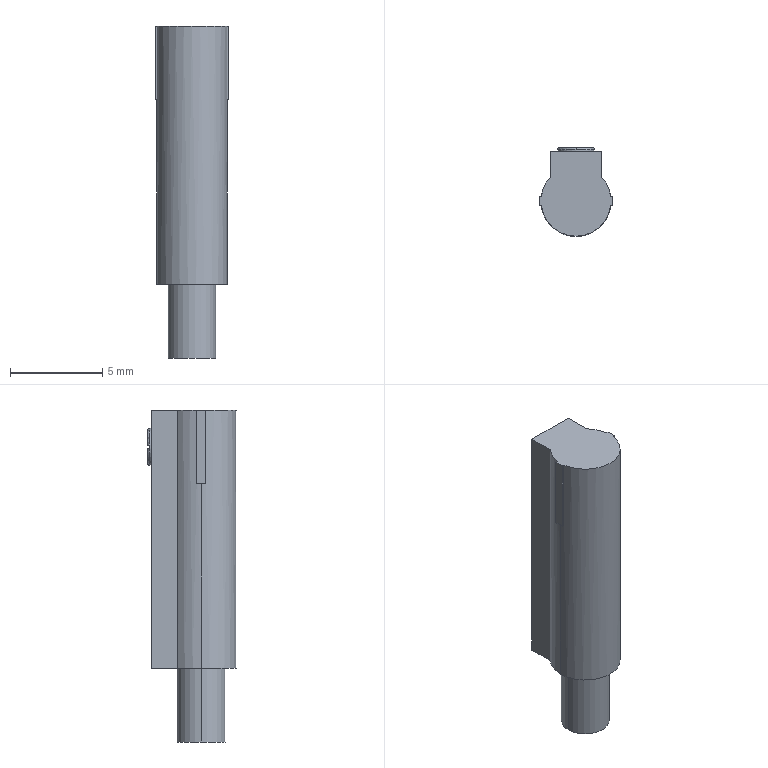Part | SolidWorks | features BaseBody 1 | 1 solid | 29 faces | box 4 x 4.8 x 18 mm | volume 219.808 mm3 | plane 19 | cylinder 7 | spline 3 | commonest cylinder face diameters 3.8 x3 2 x2 2.6 x2
STEP:
#1=CARTESIAN_POINT('',(0.8944,2.9,-1.9));
#2=VERTEX_POINT('',#1);
#3=CARTESIAN_POINT('',(0.,2.9,-1.1));
#4=VERTEX_POINT('',#3);
#5=CARTESIAN_POINT('',(0.8944,2.9,-1.9));
#6=CARTESIAN_POINT('',(0.8409,2.9,-1.421));
#7=CARTESIAN_POINT('',(0.4818,2.9,-1.1));
#8=CARTESIAN_POINT('',(0.,2.9,-1.1));
#9=(BOUNDED_CURVE()B_SPLINE_CURVE(3,(#5,#6,#7,#8),.UNSPECIFIED.,.F.,.F.)B_SPLINE_CURVE_WITH_KNOTS((4,4),(0.,0.5),.UNSPECIFIED.)CURVE()GEOMETRIC_REPRESENTATION_ITEM()RATIONAL_B_SPLINE_CURVE((1.,0.8302,0.8302,1.))REPRESENTATION_ITEM(''));
#10=EDGE_CURVE('',#2,#4,#9,.T.);
#11=ORIENTED_EDGE('',*,*,#10,.T.);
#12=CARTESIAN_POINT('',(0.,2.8,-1.));
#13=VERTEX_POINT('',#12);
#14=CARTESIAN_POINT('',(0.,2.8,-1.1));
#15=DIRECTION('',(1.,0.,0.));
#16=DIRECTION('',(0.,0.,1.));
#17=AXIS2_PLACEMENT_3D('',#14,#15,#16);
#18=CIRCLE('',#17,0.1);
#19=EDGE_CURVE('',#4,#13,#18,.T.);
#20=ORIENTED_EDGE('',*,*,#19,.T.);
#21=CARTESIAN_POINT('',(0.995,2.8,-1.9));
#22=VERTEX_POINT('',#21);
#23=CARTESIAN_POINT('',(0.,2.8,-2.));
#24=DIRECTION('',(0.,-1.,0.));
#25=DIRECTION('',(0.,0.,-1.));
#26=AXIS2_PLACEMENT_3D('',#23,#24,#25);
#27=CIRCLE('',#26,1.);
#28=EDGE_CURVE('',#22,#13,#27,.T.);
#29=ORIENTED_EDGE('',*,*,#28,.F.);
#30=CARTESIAN_POINT('',(0.995,2.8,-1.9));
#31=CARTESIAN_POINT('',(0.995,2.811,-1.9));
#32=CARTESIAN_POINT('',(0.9931,2.822,-1.9));
#33=CARTESIAN_POINT('',(0.9894,2.833,-1.9));
#34=CARTESIAN_POINT('',(0.9857,2.843,-1.9));
#35=CARTESIAN_POINT('',(0.9801,2.854,-1.9));
#36=CARTESIAN_POINT('',(0.9732,2.862,-1.9));
#37=CARTESIAN_POINT('',(0.9662,2.871,-1.9));
#38=CARTESIAN_POINT('',(0.9576,2.879,-1.9));
#39=CARTESIAN_POINT('',(0.9481,2.885,-1.9));
#40=CARTESIAN_POINT('',(0.9386,2.891,-1.9));
#41=CARTESIAN_POINT('',(0.928,2.895,-1.9));
#42=CARTESIAN_POINT('',(0.917,2.897,-1.9));
#43=CARTESIAN_POINT('',(0.9096,2.899,-1.9));
#44=CARTESIAN_POINT('',(0.902,2.9,-1.9));
#45=CARTESIAN_POINT('',(0.8944,2.9,-1.9));
#46=B_SPLINE_CURVE_WITH_KNOTS('',3,(#30,#31,#32,#33,#34,#35,#36,#37,#38,#39,#40,#41,#42,#43,#44,#45),.UNSPECIFIED.,.F.,.F.,(4,3,3,3,3,4),(0.,0.00003345,0.00006689,0.0001004,0.0001341,0.0001567),.UNSPECIFIED.);
#47=EDGE_CURVE('',#22,#2,#46,.T.);
#48=ORIENTED_EDGE('',*,*,#47,.T.);
#49=EDGE_LOOP('',(#11,#20,#29,#48));
#50=FACE_OUTER_BOUND('',#49,.T.);
#51=CARTESIAN_POINT('',(0.,2.9,-1.1));
#52=CARTESIAN_POINT('',(0.4898,2.9,-1.1));
#53=CARTESIAN_POINT('',(0.8516,2.9,-1.43));
#54=CARTESIAN_POINT('',(0.8962,2.9,-1.918));
#55=CARTESIAN_POINT('',(0.,2.9,-1.041));
#56=CARTESIAN_POINT('',(0.5217,2.9,-1.041));
#57=CARTESIAN_POINT('',(0.907,2.9,-1.393));
#58=CARTESIAN_POINT('',(0.9546,2.9,-1.913));
#59=CARTESIAN_POINT('',(0.,2.859,-1.));
#60=CARTESIAN_POINT('',(0.5442,2.859,-1.));
#61=CARTESIAN_POINT('',(0.9462,2.859,-1.367));
#62=CARTESIAN_POINT('',(0.9958,2.859,-1.909));
#63=CARTESIAN_POINT('',(0.,2.8,-1.));
#64=CARTESIAN_POINT('',(0.5442,2.8,-1.));
#65=CARTESIAN_POINT('',(0.9462,2.8,-1.367));
#66=CARTESIAN_POINT('',(0.9958,2.8,-1.909));
#67=(BOUNDED_SURFACE()B_SPLINE_SURFACE(3,3,((#51,#52,#53,#54),(#55,#56,#57,#58),(#59,#60,#61,#62),(#63,#64,#65,#66)),.UNSPECIFIED.,.F.,.F.,.F.)B_SPLINE_SURFACE_WITH_KNOTS((4,4),(4,4),(0.,1.),(0.,1.),.UNSPECIFIED.)GEOMETRIC_REPRESENTATION_ITEM()RATIONAL_B_SPLINE_SURFACE(((1.,0.8258,0.8258,1.),(0.8047,0.6645,0.6645,0.8047),(0.8047,0.6645,0.6645,0.8047),(1.,0.8258,0.8258,1.)))REPRESENTATION_ITEM('')SURFACE());
#68=ADVANCED_FACE('',(#50),#67,.T.);
#69=CARTESIAN_POINT('',(1.883,0.25,-4.));
#70=VERTEX_POINT('',#69);
#71=CARTESIAN_POINT('',(1.9,0.,-4.));
#72=VERTEX_POINT('',#71);
#73=CARTESIAN_POINT('',(0.,0.,-4.));
#74=DIRECTION('',(0.,0.,-1.));
#75=DIRECTION('',(-1.,0.,0.));
#76=AXIS2_PLACEMENT_3D('',#73,#74,#75);
#77=CIRCLE('',#76,1.9);
#78=EDGE_CURVE('',#70,#72,#77,.T.);
#79=ORIENTED_EDGE('',*,*,#78,.T.);
#80=CARTESIAN_POINT('',(1.9,0.,-14.));
#81=VERTEX_POINT('',#80);
#82=CARTESIAN_POINT('',(1.9,0.,-14.));
#83=DIRECTION('',(0.,0.,-1.));
#84=VECTOR('',#83,1000.);
#85=LINE('',#82,#84);
#86=EDGE_CURVE('',#72,#81,#85,.T.);
#87=ORIENTED_EDGE('',*,*,#86,.T.);
#88=CARTESIAN_POINT('',(1.4,1.285,-14.));
#89=VERTEX_POINT('',#88);
#90=CARTESIAN_POINT('',(0.,0.,-14.));
#91=DIRECTION('',(0.,0.,1.));
#92=DIRECTION('',(-1.,0.,0.));
#93=AXIS2_PLACEMENT_3D('',#90,#91,#92);
#94=CIRCLE('',#93,1.9);
#95=EDGE_CURVE('',#81,#89,#94,.T.);
#96=ORIENTED_EDGE('',*,*,#95,.T.);
#97=CARTESIAN_POINT('',(1.4,1.285,0.));
#98=VERTEX_POINT('',#97);
#99=CARTESIAN_POINT('',(1.4,1.285,-14.));
#100=DIRECTION('',(0.,0.,1.));
#101=VECTOR('',#100,1000.);
#102=LINE('',#99,#101);
#103=EDGE_CURVE('',#89,#98,#102,.T.);
#104=ORIENTED_EDGE('',*,*,#103,.T.);
#105=CARTESIAN_POINT('',(1.883,0.25,0.));
#106=VERTEX_POINT('',#105);
#107=CARTESIAN_POINT('',(0.,0.,0.));
#108=DIRECTION('',(0.,0.,-1.));
#109=DIRECTION('',(-1.,0.,0.));
#110=AXIS2_PLACEMENT_3D('',#107,#108,#109);
#111=CIRCLE('',#110,1.9);
#112=EDGE_CURVE('',#98,#106,#111,.T.);
#113=ORIENTED_EDGE('',*,*,#112,.T.);
#114=CARTESIAN_POINT('',(1.883,0.25,-14.));
#115=DIRECTION('',(0.,0.,-1.));
#116=VECTOR('',#115,1000.);
#117=LINE('',#114,#116);
#118=EDGE_CURVE('',#106,#70,#117,.T.);
#119=ORIENTED_EDGE('',*,*,#118,.T.);
#120=EDGE_LOOP('',(#79,#87,#96,#104,#113,#119));
#121=FACE_OUTER_BOUND('',#120,.T.);
#122=CARTESIAN_POINT('',(0.,0.,-14.));
#123=DIRECTION('',(0.,0.,-1.));
#124=DIRECTION('',(-1.,0.,0.));
#125=AXIS2_PLACEMENT_3D('',#122,#123,#124);
#126=CYLINDRICAL_SURFACE('',#125,1.9);
#127=ADVANCED_FACE('',(#121),#126,.T.);
#128=ORIENTED_EDGE('',*,*,#86,.F.);
#129=CARTESIAN_POINT('',(1.883,-0.25,-4.));
#130=VERTEX_POINT('',#129);
#131=CARTESIAN_POINT('',(0.,0.,-4.));
#132=DIRECTION('',(0.,0.,-1.));
#133=DIRECTION('',(-1.,0.,0.));
#134=AXIS2_PLACEMENT_3D('',#131,#132,#133);
#135=CIRCLE('',#134,1.9);
#136=EDGE_CURVE('',#72,#130,#135,.T.);
#137=ORIENTED_EDGE('',*,*,#136,.T.);
#138=CARTESIAN_POINT('',(1.883,-0.25,0.));
#139=VERTEX_POINT('',#138);
#140=CARTESIAN_POINT('',(1.883,-0.25,-14.));
#141=DIRECTION('',(0.,0.,1.));
#142=VECTOR('',#141,1000.);
#143=LINE('',#140,#142);
#144=EDGE_CURVE('',#130,#139,#143,.T.);
#145=ORIENTED_EDGE('',*,*,#144,.T.);
#146=CARTESIAN_POINT('',(-1.883,-0.25,0.));
#147=VERTEX_POINT('',#146);
#148=CARTESIAN_POINT('',(0.,0.,0.));
#149=DIRECTION('',(0.,0.,-1.));
#150=DIRECTION('',(-1.,0.,0.));
#151=AXIS2_PLACEMENT_3D('',#148,#149,#150);
#152=CIRCLE('',#151,1.9);
#153=EDGE_CURVE('',#139,#147,#152,.T.);
#154=ORIENTED_EDGE('',*,*,#153,.T.);
#155=CARTESIAN_POINT('',(-1.883,-0.25,-4.));
#156=VERTEX_POINT('',#155);
#157=CARTESIAN_POINT('',(-1.883,-0.25,-14.));
#158=DIRECTION('',(0.,0.,-1.));
#159=VECTOR('',#158,1000.);
#160=LINE('',#157,#159);
#161=EDGE_CURVE('',#147,#156,#160,.T.);
#162=ORIENTED_EDGE('',*,*,#161,.T.);
#163=CARTESIAN_POINT('',(-1.9,0.,-4.));
#164=VERTEX_POINT('',#163);
#165=CARTESIAN_POINT('',(0.,0.,-4.));
#166=DIRECTION('',(0.,0.,-1.));
#167=DIRECTION('',(-1.,0.,0.));
#168=AXIS2_PLACEMENT_3D('',#165,#166,#167);
#169=CIRCLE('',#168,1.9);
#170=EDGE_CURVE('',#156,#164,#169,.T.);
#171=ORIENTED_EDGE('',*,*,#170,.T.);
#172=CARTESIAN_POINT('',(-1.9,0.,-14.));
#173=VERTEX_POINT('',#172);
#174=CARTESIAN_POINT('',(-1.9,0.,-14.));
#175=DIRECTION('',(0.,0.,-1.));
#176=VECTOR('',#175,1000.);
#177=LINE('',#174,#176);
#178=EDGE_CURVE('',#164,#173,#177,.T.);
#179=ORIENTED_EDGE('',*,*,#178,.T.);
#180=CARTESIAN_POINT('',(0.,0.,-14.));
#181=DIRECTION('',(0.,0.,1.));
#182=DIRECTION('',(-1.,0.,0.));
#183=AXIS2_PLACEMENT_3D('',#180,#181,#182);
#184=CIRCLE('',#183,1.9);
#185=EDGE_CURVE('',#173,#81,#184,.T.);
#186=ORIENTED_EDGE('',*,*,#185,.T.);
#187=EDGE_LOOP('',(#128,#137,#145,#154,#162,#171,#179,#186));
#188=FACE_OUTER_BOUND('',#187,.T.);
#189=CARTESIAN_POINT('',(0.,0.,-14.));
#190=DIRECTION('',(0.,0.,-1.));
#191=DIRECTION('',(-1.,0.,0.));
#192=AXIS2_PLACEMENT_3D('',#189,#190,#191);
#193=CYLINDRICAL_SURFACE('',#192,1.9);
#194=ADVANCED_FACE('',(#188),#193,.T.);
#195=CARTESIAN_POINT('',(-1.3,0.,-14.));
#196=VERTEX_POINT('',#195);
#197=CARTESIAN_POINT('',(1.3,0.,-14.));
#198=VERTEX_POINT('',#197);
#199=CARTESIAN_POINT('',(0.,0.,-14.));
#200=DIRECTION('',(0.,0.,-1.));
#201=DIRECTION('',(-1.,0.,0.));
#202=AXIS2_PLACEMENT_3D('',#199,#200,#201);
#203=CIRCLE('',#202,1.3);
#204=EDGE_CURVE('',#196,#198,#203,.T.);
#205=ORIENTED_EDGE('',*,*,#204,.T.);
#206=CARTESIAN_POINT('',(1.3,0.,-18.));
#207=VERTEX_POINT('',#206);
#208=CARTESIAN_POINT('',(1.3,0.,-18.));
#209=DIRECTION('',(0.,0.,-1.));
#210=VECTOR('',#209,1000.);
#211=LINE('',#208,#210);
#212=EDGE_CURVE('',#198,#207,#211,.T.);
#213=ORIENTED_EDGE('',*,*,#212,.T.);
#214=CARTESIAN_POINT('',(-1.3,0.,-18.));
#215=VERTEX_POINT('',#214);
#216=CARTESIAN_POINT('',(0.,0.,-18.));
#217=DIRECTION('',(0.,0.,1.));
#218=DIRECTION('',(-1.,0.,0.));
#219=AXIS2_PLACEMENT_3D('',#216,#217,#218);
#220=CIRCLE('',#219,1.3);
#221=EDGE_CURVE('',#207,#215,#220,.T.);
#222=ORIENTED_EDGE('',*,*,#221,.T.);
#223=CARTESIAN_POINT('',(-1.3,0.,-18.));
#224=DIRECTION('',(0.,0.,-1.));
#225=VECTOR('',#224,1000.);
#226=LINE('',#223,#225);
#227=EDGE_CURVE('',#196,#215,#226,.T.);
#228=ORIENTED_EDGE('',*,*,#227,.F.);
#229=EDGE_LOOP('',(#205,#213,#222,#228));
#230=FACE_OUTER_BOUND('',#229,.T.);
#231=CARTESIAN_POINT('',(0.,0.,-18.));
#232=DIRECTION('',(0.,0.,-1.));
#233=DIRECTION('',(-1.,0.,0.));
#234=AXIS2_PLACEMENT_3D('',#231,#232,#233);
#235=CYLINDRICAL_SURFACE('',#234,1.3);
#236=ADVANCED_FACE('',(#230),#235,.T.);
#237=ORIENTED_EDGE('',*,*,#28,.T.);
#238=CARTESIAN_POINT('',(0.,2.7,-1.));
#239=VERTEX_POINT('',#238);
#240=CARTESIAN_POINT('',(0.,2.9,-1.));
#241=DIRECTION('',(0.,-1.,0.));
#242=VECTOR('',#241,1000.);
#243=LINE('',#240,#242);
#244=EDGE_CURVE('',#13,#239,#243,.T.);
#245=ORIENTED_EDGE('',*,*,#244,.T.);
#246=CARTESIAN_POINT('',(0.,2.7,-3.));
#247=VERTEX_POINT('',#246);
#248=CARTESIAN_POINT('',(0.,2.7,-2.));
#249=DIRECTION('',(0.,-1.,0.));
#250=DIRECTION('',(0.,0.,-1.));
#251=AXIS2_PLACEMENT_3D('',#248,#249,#250);
#252=CIRCLE('',#251,1.);
#253=EDGE_CURVE('',#247,#239,#252,.T.);
#254=ORIENTED_EDGE('',*,*,#253,.F.);
#255=CARTESIAN_POINT('',(0.,2.8,-3.));
#256=VERTEX_POINT('',#255);
#257=CARTESIAN_POINT('',(0.,2.9,-3.));
#258=DIRECTION('',(0.,-1.,0.));
#259=VECTOR('',#258,1000.);
#260=LINE('',#257,#259);
#261=EDGE_CURVE('',#256,#247,#260,.T.);
#262=ORIENTED_EDGE('',*,*,#261,.F.);
#263=CARTESIAN_POINT('',(0.995,2.8,-2.1));
#264=VERTEX_POINT('',#263);
#265=CARTESIAN_POINT('',(0.,2.8,-2.));
#266=DIRECTION('',(0.,-1.,0.));
#267=DIRECTION('',(0.,0.,-1.));
#268=AXIS2_PLACEMENT_3D('',#265,#266,#267);
#269=CIRCLE('',#268,1.);
#270=EDGE_CURVE('',#256,#264,#269,.T.);
#271=ORIENTED_EDGE('',*,*,#270,.T.);
#272=CARTESIAN_POINT('',(0.,2.8,-2.));
#273=DIRECTION('',(0.,1.,0.));
#274=DIRECTION('',(0.,0.,-1.));
#275=AXIS2_PLACEMENT_3D('',#272,#273,#274);
#276=CIRCLE('',#275,1.);
#277=EDGE_CURVE('',#22,#264,#276,.T.);
#278=ORIENTED_EDGE('',*,*,#277,.F.);
#279=EDGE_LOOP('',(#237,#245,#254,#262,#271,#278));
#280=FACE_OUTER_BOUND('',#279,.T.);
#281=CARTESIAN_POINT('',(0.,2.9,-2.));
#282=DIRECTION('',(0.,-1.,0.));
#283=DIRECTION('',(0.,0.,-1.));
#284=AXIS2_PLACEMENT_3D('',#281,#282,#283);
#285=CYLINDRICAL_SURFACE('',#284,1.);
#286=ADVANCED_FACE('',(#280),#285,.T.);
#287=ORIENTED_EDGE('',*,*,#178,.F.);
#288=CARTESIAN_POINT('',(-1.883,0.25,-4.));
#289=VERTEX_POINT('',#288);
#290=CARTESIAN_POINT('',(0.,0.,-4.));
#291=DIRECTION('',(0.,0.,-1.));
#292=DIRECTION('',(-1.,0.,0.));
#293=AXIS2_PLACEMENT_3D('',#290,#291,#292);
#294=CIRCLE('',#293,1.9);
#295=EDGE_CURVE('',#164,#289,#294,.T.);
#296=ORIENTED_EDGE('',*,*,#295,.T.);
#297=CARTESIAN_POINT('',(-1.883,0.25,0.));
#298=VERTEX_POINT('',#297);
#299=CARTESIAN_POINT('',(-1.883,0.25,-14.));
#300=DIRECTION('',(0.,0.,1.));
#301=VECTOR('',#300,1000.);
#302=LINE('',#299,#301);
#303=EDGE_CURVE('',#289,#298,#302,.T.);
#304=ORIENTED_EDGE('',*,*,#303,.T.);
#305=CARTESIAN_POINT('',(-1.4,1.285,0.));
#306=VERTEX_POINT('',#305);
#307=CARTESIAN_POINT('',(0.,0.,0.));
#308=DIRECTION('',(0.,0.,-1.));
#309=DIRECTION('',(-1.,0.,0.));
#310=AXIS2_PLACEMENT_3D('',#307,#308,#309);
#311=CIRCLE('',#310,1.9);
#312=EDGE_CURVE('',#298,#306,#311,.T.);
#313=ORIENTED_EDGE('',*,*,#312,.T.);
#314=CARTESIAN_POINT('',(-1.4,1.285,-14.));
#315=VERTEX_POINT('',#314);
#316=CARTESIAN_POINT('',(-1.4,1.285,-14.));
#317=DIRECTION('',(0.,0.,-1.));
#318=VECTOR('',#317,1000.);
#319=LINE('',#316,#318);
#320=EDGE_CURVE('',#306,#315,#319,.T.);
#321=ORIENTED_EDGE('',*,*,#320,.T.);
#322=CARTESIAN_POINT('',(0.,0.,-14.));
#323=DIRECTION('',(0.,0.,1.));
#324=DIRECTION('',(-1.,0.,0.));
#325=AXIS2_PLACEMENT_3D('',#322,#323,#324);
#326=CIRCLE('',#325,1.9);
#327=EDGE_CURVE('',#315,#173,#326,.T.);
#328=ORIENTED_EDGE('',*,*,#327,.T.);
#329=EDGE_LOOP('',(#287,#296,#304,#313,#321,#328));
#330=FACE_OUTER_BOUND('',#329,.T.);
#331=CARTESIAN_POINT('',(0.,0.,-14.));
#332=DIRECTION('',(0.,0.,-1.));
#333=DIRECTION('',(-1.,0.,0.));
#334=AXIS2_PLACEMENT_3D('',#331,#332,#333);
#335=CYLINDRICAL_SURFACE('',#334,1.9);
#336=ADVANCED_FACE('',(#330),#335,.T.);
#337=CARTESIAN_POINT('',(1.4,2.7,0.));
#338=VERTEX_POINT('',#337);
#339=CARTESIAN_POINT('',(-1.4,2.7,0.));
#340=VERTEX_POINT('',#339);
#341=CARTESIAN_POINT('',(0.,2.7,0.));
#342=DIRECTION('',(-1.,0.,0.));
#343=VECTOR('',#342,1000.);
#344=LINE('',#341,#343);
#345=EDGE_CURVE('',#338,#340,#344,.T.);
#346=ORIENTED_EDGE('',*,*,#345,.T.);
#347=CARTESIAN_POINT('',(-1.4,0.,0.));
#348=DIRECTION('',(0.,-1.,0.));
#349=VECTOR('',#348,1000.);
#350=LINE('',#347,#349);
#351=EDGE_CURVE('',#340,#306,#350,.T.);
#352=ORIENTED_EDGE('',*,*,#351,.T.);
#353=ORIENTED_EDGE('',*,*,#312,.F.);
#354=CARTESIAN_POINT('',(-2.,0.25,0.));
#355=VERTEX_POINT('',#354);
#356=CARTESIAN_POINT('',(0.,0.25,0.));
#357=DIRECTION('',(-1.,0.,0.));
#358=VECTOR('',#357,1000.);
#359=LINE('',#356,#358);
#360=EDGE_CURVE('',#298,#355,#359,.T.);
#361=ORIENTED_EDGE('',*,*,#360,.T.);
#362=CARTESIAN_POINT('',(-2.,-0.25,0.));
#363=VERTEX_POINT('',#362);
#364=CARTESIAN_POINT('',(-2.,0.25,0.));
#365=DIRECTION('',(0.,1.,0.));
#366=VECTOR('',#365,1000.);
#367=LINE('',#364,#366);
#368=EDGE_CURVE('',#363,#355,#367,.T.);
#369=ORIENTED_EDGE('',*,*,#368,.F.);
#370=CARTESIAN_POINT('',(0.,-0.25,0.));
#371=DIRECTION('',(1.,0.,0.));
#372=VECTOR('',#371,1000.);
#373=LINE('',#370,#372);
#374=EDGE_CURVE('',#363,#147,#373,.T.);
#375=ORIENTED_EDGE('',*,*,#374,.T.);
#376=ORIENTED_EDGE('',*,*,#153,.F.);
#377=CARTESIAN_POINT('',(2.,-0.25,0.));
#378=VERTEX_POINT('',#377);
#379=CARTESIAN_POINT('',(0.,-0.25,0.));
#380=DIRECTION('',(1.,0.,0.));
#381=VECTOR('',#380,1000.);
#382=LINE('',#379,#381);
#383=EDGE_CURVE('',#139,#378,#382,.T.);
#384=ORIENTED_EDGE('',*,*,#383,.T.);
#385=CARTESIAN_POINT('',(2.,0.25,0.));
#386=VERTEX_POINT('',#385);
#387=CARTESIAN_POINT('',(2.,-0.25,0.));
#388=DIRECTION('',(0.,-1.,0.));
#389=VECTOR('',#388,1000.);
#390=LINE('',#387,#389);
#391=EDGE_CURVE('',#386,#378,#390,.T.);
#392=ORIENTED_EDGE('',*,*,#391,.F.);
#393=CARTESIAN_POINT('',(0.,0.25,0.));
#394=DIRECTION('',(-1.,0.,0.));
#395=VECTOR('',#394,1000.);
#396=LINE('',#393,#395);
#397=EDGE_CURVE('',#386,#106,#396,.T.);
#398=ORIENTED_EDGE('',*,*,#397,.T.);
#399=ORIENTED_EDGE('',*,*,#112,.F.);
#400=CARTESIAN_POINT('',(1.4,0.,0.));
#401=DIRECTION('',(0.,1.,0.));
#402=VECTOR('',#401,1000.);
#403=LINE('',#400,#402);
#404=EDGE_CURVE('',#98,#338,#403,.T.);
#405=ORIENTED_EDGE('',*,*,#404,.T.);
#406=EDGE_LOOP('',(#346,#352,#353,#361,#369,#375,#376,#384,#392,#398,#399,#405));
#407=FACE_OUTER_BOUND('',#406,.T.);
#408=CARTESIAN_POINT('',(0.,0.,0.));
#409=DIRECTION('',(0.,0.,1.));
#410=DIRECTION('',(1.,0.,0.));
#411=AXIS2_PLACEMENT_3D('',#408,#409,#410);
#412=PLANE('',#411);
#413=ADVANCED_FACE('',(#407),#412,.T.);
#414=CARTESIAN_POINT('',(2.,-0.25,-4.));
#415=VERTEX_POINT('',#414);
#416=CARTESIAN_POINT('',(-2.,-0.25,-4.));
#417=DIRECTION('',(1.,0.,0.));
#418=VECTOR('',#417,1000.);
#419=LINE('',#416,#418);
#420=EDGE_CURVE('',#130,#415,#419,.T.);
#421=ORIENTED_EDGE('',*,*,#420,.T.);
#422=CARTESIAN_POINT('',(2.,-0.25,-4.));
#423=DIRECTION('',(0.,0.,1.));
#424=VECTOR('',#423,1000.);
#425=LINE('',#422,#424);
#426=EDGE_CURVE('',#415,#378,#425,.T.);
#427=ORIENTED_EDGE('',*,*,#426,.T.);
#428=ORIENTED_EDGE('',*,*,#383,.F.);
#429=ORIENTED_EDGE('',*,*,#144,.F.);
#430=EDGE_LOOP('',(#421,#427,#428,#429));
#431=FACE_OUTER_BOUND('',#430,.T.);
#432=CARTESIAN_POINT('',(-2.,-0.25,-4.));
#433=DIRECTION('',(0.,-1.,0.));
#434=DIRECTION('',(0.,0.,-1.));
#435=AXIS2_PLACEMENT_3D('',#432,#433,#434);
#436=PLANE('',#435);
#437=ADVANCED_FACE('',(#431),#436,.T.);
#438=CARTESIAN_POINT('',(2.,0.25,-4.));
#439=VERTEX_POINT('',#438);
#440=CARTESIAN_POINT('',(0.,0.25,-4.));
#441=DIRECTION('',(-1.,0.,0.));
#442=VECTOR('',#441,1000.);
#443=LINE('',#440,#442);
#444=EDGE_CURVE('',#439,#70,#443,.T.);
#445=ORIENTED_EDGE('',*,*,#444,.F.);
#446=CARTESIAN_POINT('',(2.,0.,-4.));
#447=DIRECTION('',(0.,1.,0.));
#448=VECTOR('',#447,1000.);
#449=LINE('',#446,#448);
#450=EDGE_CURVE('',#415,#439,#449,.T.);
#451=ORIENTED_EDGE('',*,*,#450,.F.);
#452=ORIENTED_EDGE('',*,*,#420,.F.);
#453=ORIENTED_EDGE('',*,*,#136,.F.);
#454=ORIENTED_EDGE('',*,*,#78,.F.);
#455=EDGE_LOOP('',(#445,#451,#452,#453,#454));
#456=FACE_OUTER_BOUND('',#455,.T.);
#457=CARTESIAN_POINT('',(0.,0.,-4.));
#458=DIRECTION('',(0.,0.,1.));
#459=DIRECTION('',(1.,0.,0.));
#460=AXIS2_PLACEMENT_3D('',#457,#458,#459);
#461=PLANE('',#460);
#462=ADVANCED_FACE('',(#456),#461,.F.);
#463=ORIENTED_EDGE('',*,*,#397,.F.);
#464=CARTESIAN_POINT('',(2.,0.25,-4.));
#465=DIRECTION('',(0.,0.,-1.));
#466=VECTOR('',#465,1000.);
#467=LINE('',#464,#466);
#468=EDGE_CURVE('',#386,#439,#467,.T.);
#469=ORIENTED_EDGE('',*,*,#468,.T.);
#470=ORIENTED_EDGE('',*,*,#444,.T.);
#471=ORIENTED_EDGE('',*,*,#118,.F.);
#472=EDGE_LOOP('',(#463,#469,#470,#471));
#473=FACE_OUTER_BOUND('',#472,.T.);
#474=CARTESIAN_POINT('',(2.,0.25,-4.));
#475=DIRECTION('',(0.,1.,0.));
#476=DIRECTION('',(0.,0.,1.));
#477=AXIS2_PLACEMENT_3D('',#474,#475,#476);
#478=PLANE('',#477);
#479=ADVANCED_FACE('',(#473),#478,.T.);
#480=CARTESIAN_POINT('',(1.4,2.7,-14.));
#481=VERTEX_POINT('',#480);
#482=CARTESIAN_POINT('',(1.4,1.285,-14.));
#483=DIRECTION('',(0.,1.,0.));
#484=VECTOR('',#483,1000.);
#485=LINE('',#482,#484);
#486=EDGE_CURVE('',#89,#481,#485,.T.);
#487=ORIENTED_EDGE('',*,*,#486,.T.);
#488=CARTESIAN_POINT('',(1.4,2.7,-14.));
#489=DIRECTION('',(0.,0.,1.));
#490=VECTOR('',#489,1000.);
#491=LINE('',#488,#490);
#492=EDGE_CURVE('',#481,#338,#491,.T.);
#493=ORIENTED_EDGE('',*,*,#492,.T.);
#494=ORIENTED_EDGE('',*,*,#404,.F.);
#495=ORIENTED_EDGE('',*,*,#103,.F.);
#496=EDGE_LOOP('',(#487,#493,#494,#495));
#497=FACE_OUTER_BOUND('',#496,.T.);
#498=CARTESIAN_POINT('',(1.4,1.285,-14.));
#499=DIRECTION('',(1.,0.,0.));
#500=DIRECTION('',(0.,0.,-1.));
#501=AXIS2_PLACEMENT_3D('',#498,#499,#500);
#502=PLANE('',#501);
#503=ADVANCED_FACE('',(#497),#502,.T.);
#504=CARTESIAN_POINT('',(-1.4,2.7,-14.));
#505=VERTEX_POINT('',#504);
#506=CARTESIAN_POINT('',(0.,2.7,-14.));
#507=DIRECTION('',(-1.,0.,0.));
#508=VECTOR('',#507,1000.);
#509=LINE('',#506,#508);
#510=EDGE_CURVE('',#481,#505,#509,.T.);
#511=ORIENTED_EDGE('',*,*,#510,.F.);
#512=ORIENTED_EDGE('',*,*,#486,.F.);
#513=ORIENTED_EDGE('',*,*,#95,.F.);
#514=ORIENTED_EDGE('',*,*,#185,.F.);
#515=ORIENTED_EDGE('',*,*,#327,.F.);
#516=CARTESIAN_POINT('',(-1.4,0.,-14.));
#517=DIRECTION('',(0.,-1.,0.));
#518=VECTOR('',#517,1000.);
#519=LINE('',#516,#518);
#520=EDGE_CURVE('',#505,#315,#519,.T.);
#521=ORIENTED_EDGE('',*,*,#520,.F.);
#522=EDGE_LOOP('',(#511,#512,#513,#514,#515,#521));
#523=FACE_OUTER_BOUND('',#522,.T.);
#524=ORIENTED_EDGE('',*,*,#204,.F.);
#525=CARTESIAN_POINT('',(0.,0.,-14.));
#526=DIRECTION('',(0.,0.,-1.));
#527=DIRECTION('',(-1.,0.,0.));
#528=AXIS2_PLACEMENT_3D('',#525,#526,#527);
#529=CIRCLE('',#528,1.3);
#530=EDGE_CURVE('',#198,#196,#529,.T.);
#531=ORIENTED_EDGE('',*,*,#530,.F.);
#532=EDGE_LOOP('',(#524,#531));
#533=FACE_BOUND('',#532,.T.);
#534=CARTESIAN_POINT('',(0.,0.,-14.));
#535=DIRECTION('',(0.,0.,1.));
#536=DIRECTION('',(1.,0.,0.));
#537=AXIS2_PLACEMENT_3D('',#534,#535,#536);
#538=PLANE('',#537);
#539=ADVANCED_FACE('',(#523,#533),#538,.F.);
#540=ORIENTED_EDGE('',*,*,#520,.T.);
#541=ORIENTED_EDGE('',*,*,#320,.F.);
#542=ORIENTED_EDGE('',*,*,#351,.F.);
#543=CARTESIAN_POINT('',(-1.4,2.7,-14.));
#544=DIRECTION('',(0.,0.,-1.));
#545=VECTOR('',#544,1000.);
#546=LINE('',#543,#545);
#547=EDGE_CURVE('',#340,#505,#546,.T.);
#548=ORIENTED_EDGE('',*,*,#547,.T.);
#549=EDGE_LOOP('',(#540,#541,#542,#548));
#550=FACE_OUTER_BOUND('',#549,.T.);
#551=CARTESIAN_POINT('',(-1.4,2.7,-14.));
#552=DIRECTION('',(-1.,0.,0.));
#553=DIRECTION('',(0.,0.,1.));
#554=AXIS2_PLACEMENT_3D('',#551,#552,#553);
#555=PLANE('',#554);
#556=ADVANCED_FACE('',(#550),#555,.T.);
#557=CARTESIAN_POINT('',(-2.,0.25,-4.));
#558=VERTEX_POINT('',#557);
#559=CARTESIAN_POINT('',(2.,0.25,-4.));
#560=DIRECTION('',(-1.,0.,0.));
#561=VECTOR('',#560,1000.);
#562=LINE('',#559,#561);
#563=EDGE_CURVE('',#289,#558,#562,.T.);
#564=ORIENTED_EDGE('',*,*,#563,.T.);
#565=CARTESIAN_POINT('',(-2.,0.25,-4.));
#566=DIRECTION('',(0.,0.,1.));
#567=VECTOR('',#566,1000.);
#568=LINE('',#565,#567);
#569=EDGE_CURVE('',#558,#355,#568,.T.);
#570=ORIENTED_EDGE('',*,*,#569,.T.);
#571=ORIENTED_EDGE('',*,*,#360,.F.);
#572=ORIENTED_EDGE('',*,*,#303,.F.);
#573=EDGE_LOOP('',(#564,#570,#571,#572));
#574=FACE_OUTER_BOUND('',#573,.T.);
#575=CARTESIAN_POINT('',(2.,0.25,-4.));
#576=DIRECTION('',(0.,1.,0.));
#577=DIRECTION('',(0.,0.,1.));
#578=AXIS2_PLACEMENT_3D('',#575,#576,#577);
#579=PLANE('',#578);
#580=ADVANCED_FACE('',(#574),#579,.T.);
#581=CARTESIAN_POINT('',(-2.,-0.25,-4.));
#582=VERTEX_POINT('',#581);
#583=CARTESIAN_POINT('',(0.,-0.25,-4.));
#584=DIRECTION('',(1.,0.,0.));
#585=VECTOR('',#584,1000.);
#586=LINE('',#583,#585);
#587=EDGE_CURVE('',#582,#156,#586,.T.);
#588=ORIENTED_EDGE('',*,*,#587,.F.);
#589=CARTESIAN_POINT('',(-2.,0.,-4.));
#590=DIRECTION('',(0.,-1.,0.));
#591=VECTOR('',#590,1000.);
#592=LINE('',#589,#591);
#593=EDGE_CURVE('',#558,#582,#592,.T.);
#594=ORIENTED_EDGE('',*,*,#593,.F.);
#595=ORIENTED_EDGE('',*,*,#563,.F.);
#596=ORIENTED_EDGE('',*,*,#295,.F.);
#597=ORIENTED_EDGE('',*,*,#170,.F.);
#598=EDGE_LOOP('',(#588,#594,#595,#596,#597));
#599=FACE_OUTER_BOUND('',#598,.T.);
#600=CARTESIAN_POINT('',(0.,0.,-4.));
#601=DIRECTION('',(0.,0.,1.));
#602=DIRECTION('',(1.,0.,0.));
#603=AXIS2_PLACEMENT_3D('',#600,#601,#602);
#604=PLANE('',#603);
#605=ADVANCED_FACE('',(#599),#604,.F.);
#606=ORIENTED_EDGE('',*,*,#374,.F.);
#607=CARTESIAN_POINT('',(-2.,-0.25,-4.));
#608=DIRECTION('',(0.,0.,-1.));
#609=VECTOR('',#608,1000.);
#610=LINE('',#607,#609);
#611=EDGE_CURVE('',#363,#582,#610,.T.);
#612=ORIENTED_EDGE('',*,*,#611,.T.);
#613=ORIENTED_EDGE('',*,*,#587,.T.);
#614=ORIENTED_EDGE('',*,*,#161,.F.);
#615=EDGE_LOOP('',(#606,#612,#613,#614));
#616=FACE_OUTER_BOUND('',#615,.T.);
#617=CARTESIAN_POINT('',(-2.,-0.25,-4.));
#618=DIRECTION('',(0.,-1.,0.));
#619=DIRECTION('',(0.,0.,-1.));
#620=AXIS2_PLACEMENT_3D('',#617,#618,#619);
#621=PLANE('',#620);
#622=ADVANCED_FACE('',(#616),#621,.T.);
#623=ORIENTED_EDGE('',*,*,#510,.T.);
#624=ORIENTED_EDGE('',*,*,#547,.F.);
#625=ORIENTED_EDGE('',*,*,#345,.F.);
#626=ORIENTED_EDGE('',*,*,#492,.F.);
#627=EDGE_LOOP('',(#623,#624,#625,#626));
#628=FACE_OUTER_BOUND('',#627,.T.);
#629=ORIENTED_EDGE('',*,*,#253,.T.);
#630=CARTESIAN_POINT('',(0.,2.7,-2.));
#631=DIRECTION('',(0.,-1.,0.));
#632=DIRECTION('',(0.,0.,-1.));
#633=AXIS2_PLACEMENT_3D('',#630,#631,#632);
#634=CIRCLE('',#633,1.);
#635=EDGE_CURVE('',#239,#247,#634,.T.);
#636=ORIENTED_EDGE('',*,*,#635,.T.);
#637=EDGE_LOOP('',(#629,#636));
#638=FACE_BOUND('',#637,.T.);
#639=CARTESIAN_POINT('',(1.4,2.7,-14.));
#640=DIRECTION('',(0.,1.,0.));
#641=DIRECTION('',(0.,0.,1.));
#642=AXIS2_PLACEMENT_3D('',#639,#640,#641);
#643=PLANE('',#642);
#644=ADVANCED_FACE('',(#628,#638),#643,.T.);
#645=ORIENTED_EDGE('',*,*,#450,.T.);
#646=ORIENTED_EDGE('',*,*,#468,.F.);
#647=ORIENTED_EDGE('',*,*,#391,.T.);
#648=ORIENTED_EDGE('',*,*,#426,.F.);
#649=EDGE_LOOP('',(#645,#646,#647,#648));
#650=FACE_OUTER_BOUND('',#649,.T.);
#651=CARTESIAN_POINT('',(2.,-0.25,-4.));
#652=DIRECTION('',(1.,0.,0.));
#653=DIRECTION('',(0.,0.,-1.));
#654=AXIS2_PLACEMENT_3D('',#651,#652,#653);
#655=PLANE('',#654);
#656=ADVANCED_FACE('',(#650),#655,.T.);
#657=ORIENTED_EDGE('',*,*,#212,.F.);
#658=ORIENTED_EDGE('',*,*,#530,.T.);
#659=ORIENTED_EDGE('',*,*,#227,.T.);
#660=CARTESIAN_POINT('',(0.,0.,-18.));
#661=DIRECTION('',(0.,0.,1.));
#662=DIRECTION('',(-1.,0.,0.));
#663=AXIS2_PLACEMENT_3D('',#660,#661,#662);
#664=CIRCLE('',#663,1.3);
#665=EDGE_CURVE('',#215,#207,#664,.T.);
#666=ORIENTED_EDGE('',*,*,#665,.T.);
#667=EDGE_LOOP('',(#657,#658,#659,#666));
#668=FACE_OUTER_BOUND('',#667,.T.);
#669=CARTESIAN_POINT('',(0.,0.,-18.));
#670=DIRECTION('',(0.,0.,-1.));
#671=DIRECTION('',(-1.,0.,0.));
#672=AXIS2_PLACEMENT_3D('',#669,#670,#671);
#673=CYLINDRICAL_SURFACE('',#672,1.3);
#674=ADVANCED_FACE('',(#668),#673,.T.);
#675=ORIENTED_EDGE('',*,*,#593,.T.);
#676=ORIENTED_EDGE('',*,*,#611,.F.);
#677=ORIENTED_EDGE('',*,*,#368,.T.);
#678=ORIENTED_EDGE('',*,*,#569,.F.);
#679=EDGE_LOOP('',(#675,#676,#677,#678));
#680=FACE_OUTER_BOUND('',#679,.T.);
#681=CARTESIAN_POINT('',(-2.,0.25,-4.));
#682=DIRECTION('',(-1.,0.,0.));
#683=DIRECTION('',(0.,0.,1.));
#684=AXIS2_PLACEMENT_3D('',#681,#682,#683);
#685=PLANE('',#684);
#686=ADVANCED_FACE('',(#680),#685,.T.);
#687=ORIENTED_EDGE('',*,*,#244,.F.);
#688=CARTESIAN_POINT('',(-0.995,2.8,-1.9));
#689=VERTEX_POINT('',#688);
#690=CARTESIAN_POINT('',(0.,2.8,-2.));
#691=DIRECTION('',(0.,-1.,0.));
#692=DIRECTION('',(0.,0.,-1.));
#693=AXIS2_PLACEMENT_3D('',#690,#691,#692);
#694=CIRCLE('',#693,1.);
#695=EDGE_CURVE('',#13,#689,#694,.T.);
#696=ORIENTED_EDGE('',*,*,#695,.T.);
#697=CARTESIAN_POINT('',(-0.995,2.8,-2.1));
#698=VERTEX_POINT('',#697);
#699=CARTESIAN_POINT('',(0.,2.8,-2.));
#700=DIRECTION('',(0.,1.,0.));
#701=DIRECTION('',(0.,0.,-1.));
#702=AXIS2_PLACEMENT_3D('',#699,#700,#701);
#703=CIRCLE('',#702,1.);
#704=EDGE_CURVE('',#698,#689,#703,.T.);
#705=ORIENTED_EDGE('',*,*,#704,.F.);
#706=CARTESIAN_POINT('',(0.,2.8,-2.));
#707=DIRECTION('',(0.,-1.,0.));
#708=DIRECTION('',(0.,0.,-1.));
#709=AXIS2_PLACEMENT_3D('',#706,#707,#708);
#710=CIRCLE('',#709,1.);
#711=EDGE_CURVE('',#698,#256,#710,.T.);
#712=ORIENTED_EDGE('',*,*,#711,.T.);
#713=ORIENTED_EDGE('',*,*,#261,.T.);
#714=ORIENTED_EDGE('',*,*,#635,.F.);
#715=EDGE_LOOP('',(#687,#696,#705,#712,#713,#714));
#716=FACE_OUTER_BOUND('',#715,.T.);
#717=CARTESIAN_POINT('',(0.,2.9,-2.));
#718=DIRECTION('',(0.,-1.,0.));
#719=DIRECTION('',(0.,0.,-1.));
#720=AXIS2_PLACEMENT_3D('',#717,#718,#719);
#721=CYLINDRICAL_SURFACE('',#720,1.);
#722=ADVANCED_FACE('',(#716),#721,.T.);
#723=ORIENTED_EDGE('',*,*,#665,.F.);
#724=ORIENTED_EDGE('',*,*,#221,.F.);
#725=EDGE_LOOP('',(#723,#724));
#726=FACE_OUTER_BOUND('',#725,.T.);
#727=CARTESIAN_POINT('',(0.,0.,-18.));
#728=DIRECTION('',(0.,0.,1.));
#729=DIRECTION('',(1.,0.,0.));
#730=AXIS2_PLACEMENT_3D('',#727,#728,#729);
#731=PLANE('',#730);
#732=ADVANCED_FACE('',(#726),#731,.F.);
#733=CARTESIAN_POINT('',(0.8944,2.9,-2.1));
#734=VERTEX_POINT('',#733);
#735=CARTESIAN_POINT('',(0.8944,2.9,-2.1));
#736=CARTESIAN_POINT('',(0.9057,2.9,-2.1));
#737=CARTESIAN_POINT('',(0.9172,2.898,-2.1));
#738=CARTESIAN_POINT('',(0.9279,2.894,-2.1));
#739=CARTESIAN_POINT('',(0.9385,2.891,-2.1));
#740=CARTESIAN_POINT('',(0.9487,2.885,-2.1));
#741=CARTESIAN_POINT('',(0.9575,2.878,-2.1));
#742=CARTESIAN_POINT('',(0.9663,2.871,-2.1));
#743=CARTESIAN_POINT('',(0.974,2.862,-2.1));
#744=CARTESIAN_POINT('',(0.98,2.853,-2.1));
#745=CARTESIAN_POINT('',(0.9859,2.843,-2.1));
#746=CARTESIAN_POINT('',(0.9902,2.832,-2.1));
#747=CARTESIAN_POINT('',(0.9927,2.821,-2.1));
#748=CARTESIAN_POINT('',(0.9942,2.814,-2.1));
#749=CARTESIAN_POINT('',(0.995,2.807,-2.1));
#750=CARTESIAN_POINT('',(0.995,2.8,-2.1));
#751=B_SPLINE_CURVE_WITH_KNOTS('',3,(#735,#736,#737,#738,#739,#740,#741,#742,#743,#744,#745,#746,#747,#748,#749,#750),.UNSPECIFIED.,.F.,.F.,(4,3,3,3,3,4),(0.,0.00003392,0.00006784,0.0001017,0.0001353,0.0001567),.UNSPECIFIED.);
#752=EDGE_CURVE('',#734,#264,#751,.T.);
#753=ORIENTED_EDGE('',*,*,#752,.T.);
#754=ORIENTED_EDGE('',*,*,#270,.F.);
#755=ORIENTED_EDGE('',*,*,#711,.F.);
#756=CARTESIAN_POINT('',(-0.8944,2.9,-2.1));
#757=VERTEX_POINT('',#756);
#758=CARTESIAN_POINT('',(-0.995,2.8,-2.1));
#759=CARTESIAN_POINT('',(-0.995,2.811,-2.1));
#760=CARTESIAN_POINT('',(-0.9931,2.822,-2.1));
#761=CARTESIAN_POINT('',(-0.9894,2.833,-2.1));
#762=CARTESIAN_POINT('',(-0.9857,2.843,-2.1));
#763=CARTESIAN_POINT('',(-0.9801,2.854,-2.1));
#764=CARTESIAN_POINT('',(-0.9732,2.862,-2.1));
#765=CARTESIAN_POINT('',(-0.9662,2.871,-2.1));
#766=CARTESIAN_POINT('',(-0.9576,2.879,-2.1));
#767=CARTESIAN_POINT('',(-0.9481,2.885,-2.1));
#768=CARTESIAN_POINT('',(-0.9386,2.891,-2.1));
#769=CARTESIAN_POINT('',(-0.928,2.895,-2.1));
#770=CARTESIAN_POINT('',(-0.917,2.897,-2.1));
#771=CARTESIAN_POINT('',(-0.9096,2.899,-2.1));
#772=CARTESIAN_POINT('',(-0.902,2.9,-2.1));
#773=CARTESIAN_POINT('',(-0.8944,2.9,-2.1));
#774=B_SPLINE_CURVE_WITH_KNOTS('',3,(#758,#759,#760,#761,#762,#763,#764,#765,#766,#767,#768,#769,#770,#771,#772,#773),.UNSPECIFIED.,.F.,.F.,(4,3,3,3,3,4),(0.,0.00003345,0.00006689,0.0001004,0.0001341,0.0001567),.UNSPECIFIED.);
#775=EDGE_CURVE('',#698,#757,#774,.T.);
#776=ORIENTED_EDGE('',*,*,#775,.T.);
#777=CARTESIAN_POINT('',(-0.8944,2.9,-2.1));
#778=CARTESIAN_POINT('',(-0.7318,2.9,-3.555));
#779=CARTESIAN_POINT('',(0.7318,2.9,-3.555));
#780=CARTESIAN_POINT('',(0.8944,2.9,-2.1));
#781=(BOUNDED_CURVE()B_SPLINE_CURVE(3,(#777,#778,#779,#780),.UNSPECIFIED.,.F.,.T.)B_SPLINE_CURVE_WITH_KNOTS((4,4),(0.,1.),.UNSPECIFIED.)CURVE()GEOMETRIC_REPRESENTATION_ITEM()RATIONAL_B_SPLINE_CURVE((1.,0.4074,0.4074,1.))REPRESENTATION_ITEM(''));
#782=EDGE_CURVE('',#757,#734,#781,.T.);
#783=ORIENTED_EDGE('',*,*,#782,.T.);
#784=EDGE_LOOP('',(#753,#754,#755,#776,#783));
#785=FACE_OUTER_BOUND('',#784,.T.);
#786=CARTESIAN_POINT('',(0.8969,2.9,-2.074));
#787=CARTESIAN_POINT('',(0.77,2.9,-3.609));
#788=CARTESIAN_POINT('',(-0.77,2.9,-3.609));
#789=CARTESIAN_POINT('',(-0.8969,2.9,-2.074));
#790=CARTESIAN_POINT('',(0.9553,2.9,-2.079));
#791=CARTESIAN_POINT('',(0.8201,2.9,-3.714));
#792=CARTESIAN_POINT('',(-0.8201,2.9,-3.714));
#793=CARTESIAN_POINT('',(-0.9553,2.9,-2.079));
#794=CARTESIAN_POINT('',(0.9966,2.859,-2.082));
#795=CARTESIAN_POINT('',(0.8556,2.859,-3.788));
#796=CARTESIAN_POINT('',(-0.8556,2.859,-3.788));
#797=CARTESIAN_POINT('',(-0.9966,2.859,-2.082));
#798=CARTESIAN_POINT('',(0.9966,2.8,-2.082));
#799=CARTESIAN_POINT('',(0.8556,2.8,-3.788));
#800=CARTESIAN_POINT('',(-0.8556,2.8,-3.788));
#801=CARTESIAN_POINT('',(-0.9966,2.8,-2.082));
#802=(BOUNDED_SURFACE()B_SPLINE_SURFACE(3,3,((#786,#787,#788,#789),(#790,#791,#792,#793),(#794,#795,#796,#797),(#798,#799,#800,#801)),.UNSPECIFIED.,.F.,.F.,.F.)B_SPLINE_SURFACE_WITH_KNOTS((4,4),(4,4),(0.,1.),(0.,1.),.UNSPECIFIED.)GEOMETRIC_REPRESENTATION_ITEM()RATIONAL_B_SPLINE_SURFACE(((1.,0.3883,0.3883,1.),(0.8047,0.3125,0.3125,0.8047),(0.8047,0.3125,0.3125,0.8047),(1.,0.3883,0.3883,1.)))REPRESENTATION_ITEM('')SURFACE());
#803=ADVANCED_FACE('',(#785),#802,.T.);
#804=ORIENTED_EDGE('',*,*,#19,.F.);
#805=CARTESIAN_POINT('',(-0.8944,2.9,-1.9));
#806=VERTEX_POINT('',#805);
#807=CARTESIAN_POINT('',(0.,2.9,-1.1));
#808=CARTESIAN_POINT('',(-0.4818,2.9,-1.1));
#809=CARTESIAN_POINT('',(-0.8409,2.9,-1.421));
#810=CARTESIAN_POINT('',(-0.8944,2.9,-1.9));
#811=(BOUNDED_CURVE()B_SPLINE_CURVE(3,(#807,#808,#809,#810),.UNSPECIFIED.,.F.,.F.)B_SPLINE_CURVE_WITH_KNOTS((4,4),(0.5,1.),.UNSPECIFIED.)CURVE()GEOMETRIC_REPRESENTATION_ITEM()RATIONAL_B_SPLINE_CURVE((1.,0.8302,0.8302,1.))REPRESENTATION_ITEM(''));
#812=EDGE_CURVE('',#4,#806,#811,.T.);
#813=ORIENTED_EDGE('',*,*,#812,.T.);
#814=CARTESIAN_POINT('',(-0.8944,2.9,-1.9));
#815=CARTESIAN_POINT('',(-0.9057,2.9,-1.9));
#816=CARTESIAN_POINT('',(-0.9172,2.898,-1.9));
#817=CARTESIAN_POINT('',(-0.9279,2.894,-1.9));
#818=CARTESIAN_POINT('',(-0.9385,2.891,-1.9));
#819=CARTESIAN_POINT('',(-0.9487,2.885,-1.9));
#820=CARTESIAN_POINT('',(-0.9575,2.878,-1.9));
#821=CARTESIAN_POINT('',(-0.9663,2.871,-1.9));
#822=CARTESIAN_POINT('',(-0.974,2.862,-1.9));
#823=CARTESIAN_POINT('',(-0.98,2.853,-1.9));
#824=CARTESIAN_POINT('',(-0.9859,2.843,-1.9));
#825=CARTESIAN_POINT('',(-0.9902,2.832,-1.9));
#826=CARTESIAN_POINT('',(-0.9927,2.821,-1.9));
#827=CARTESIAN_POINT('',(-0.9942,2.814,-1.9));
#828=CARTESIAN_POINT('',(-0.995,2.807,-1.9));
#829=CARTESIAN_POINT('',(-0.995,2.8,-1.9));
#830=B_SPLINE_CURVE_WITH_KNOTS('',3,(#814,#815,#816,#817,#818,#819,#820,#821,#822,#823,#824,#825,#826,#827,#828,#829),.UNSPECIFIED.,.F.,.F.,(4,3,3,3,3,4),(0.,0.00003392,0.00006784,0.0001017,0.0001353,0.0001567),.UNSPECIFIED.);
#831=EDGE_CURVE('',#806,#689,#830,.T.);
#832=ORIENTED_EDGE('',*,*,#831,.T.);
#833=ORIENTED_EDGE('',*,*,#695,.F.);
#834=EDGE_LOOP('',(#804,#813,#832,#833));
#835=FACE_OUTER_BOUND('',#834,.T.);
#836=CARTESIAN_POINT('',(-0.8962,2.9,-1.918));
#837=CARTESIAN_POINT('',(-0.8516,2.9,-1.43));
#838=CARTESIAN_POINT('',(-0.4898,2.9,-1.1));
#839=CARTESIAN_POINT('',(0.,2.9,-1.1));
#840=CARTESIAN_POINT('',(-0.9546,2.9,-1.913));
#841=CARTESIAN_POINT('',(-0.907,2.9,-1.393));
#842=CARTESIAN_POINT('',(-0.5217,2.9,-1.041));
#843=CARTESIAN_POINT('',(0.,2.9,-1.041));
#844=CARTESIAN_POINT('',(-0.9958,2.859,-1.909));
#845=CARTESIAN_POINT('',(-0.9462,2.859,-1.367));
#846=CARTESIAN_POINT('',(-0.5442,2.859,-1.));
#847=CARTESIAN_POINT('',(0.,2.859,-1.));
#848=CARTESIAN_POINT('',(-0.9958,2.8,-1.909));
#849=CARTESIAN_POINT('',(-0.9462,2.8,-1.367));
#850=CARTESIAN_POINT('',(-0.5442,2.8,-1.));
#851=CARTESIAN_POINT('',(0.,2.8,-1.));
#852=(BOUNDED_SURFACE()B_SPLINE_SURFACE(3,3,((#836,#837,#838,#839),(#840,#841,#842,#843),(#844,#845,#846,#847),(#848,#849,#850,#851)),.UNSPECIFIED.,.F.,.F.,.F.)B_SPLINE_SURFACE_WITH_KNOTS((4,4),(4,4),(0.,1.),(0.,1.),.UNSPECIFIED.)GEOMETRIC_REPRESENTATION_ITEM()RATIONAL_B_SPLINE_SURFACE(((1.,0.8258,0.8258,1.),(0.8047,0.6645,0.6645,0.8047),(0.8047,0.6645,0.6645,0.8047),(1.,0.8258,0.8258,1.)))REPRESENTATION_ITEM('')SURFACE());
#853=ADVANCED_FACE('',(#835),#852,.T.);
#854=CARTESIAN_POINT('',(0.,2.9,-2.1));
#855=DIRECTION('',(-1.,0.,0.));
#856=VECTOR('',#855,1000.);
#857=LINE('',#854,#856);
#858=EDGE_CURVE('',#734,#757,#857,.T.);
#859=ORIENTED_EDGE('',*,*,#858,.F.);
#860=ORIENTED_EDGE('',*,*,#782,.F.);
#861=EDGE_LOOP('',(#859,#860));
#862=FACE_OUTER_BOUND('',#861,.T.);
#863=CARTESIAN_POINT('',(0.,2.9,-1.1));
#864=DIRECTION('',(0.,-1.,0.));
#865=DIRECTION('',(0.,0.,-1.));
#866=AXIS2_PLACEMENT_3D('',#863,#864,#865);
#867=PLANE('',#866);
#868=ADVANCED_FACE('',(#862),#867,.F.);
#869=ORIENTED_EDGE('',*,*,#10,.F.);
#870=CARTESIAN_POINT('',(0.,2.9,-1.9));
#871=DIRECTION('',(1.,0.,0.));
#872=VECTOR('',#871,1000.);
#873=LINE('',#870,#872);
#874=EDGE_CURVE('',#806,#2,#873,.T.);
#875=ORIENTED_EDGE('',*,*,#874,.F.);
#876=ORIENTED_EDGE('',*,*,#812,.F.);
#877=EDGE_LOOP('',(#869,#875,#876));
#878=FACE_OUTER_BOUND('',#877,.T.);
#879=CARTESIAN_POINT('',(0.,2.9,-1.1));
#880=DIRECTION('',(0.,-1.,0.));
#881=DIRECTION('',(0.,0.,-1.));
#882=AXIS2_PLACEMENT_3D('',#879,#880,#881);
#883=PLANE('',#882);
#884=ADVANCED_FACE('',(#878),#883,.F.);
#885=CARTESIAN_POINT('',(1.,2.8,-2.1));
#886=DIRECTION('',(-1.,0.,0.));
#887=VECTOR('',#886,1000.);
#888=LINE('',#885,#887);
#889=EDGE_CURVE('',#264,#698,#888,.T.);
#890=ORIENTED_EDGE('',*,*,#889,.F.);
#891=ORIENTED_EDGE('',*,*,#752,.F.);
#892=ORIENTED_EDGE('',*,*,#858,.T.);
#893=ORIENTED_EDGE('',*,*,#775,.F.);
#894=EDGE_LOOP('',(#890,#891,#892,#893));
#895=FACE_OUTER_BOUND('',#894,.T.);
#896=CARTESIAN_POINT('',(1.,2.8,-2.1));
#897=DIRECTION('',(0.,0.,-1.));
#898=DIRECTION('',(-1.,0.,0.));
#899=AXIS2_PLACEMENT_3D('',#896,#897,#898);
#900=PLANE('',#899);
#901=ADVANCED_FACE('',(#895),#900,.F.);
#902=ORIENTED_EDGE('',*,*,#874,.T.);
#903=ORIENTED_EDGE('',*,*,#47,.F.);
#904=CARTESIAN_POINT('',(-1.,2.8,-1.9));
#905=DIRECTION('',(1.,0.,0.));
#906=VECTOR('',#905,1000.);
#907=LINE('',#904,#906);
#908=EDGE_CURVE('',#689,#22,#907,.T.);
#909=ORIENTED_EDGE('',*,*,#908,.F.);
#910=ORIENTED_EDGE('',*,*,#831,.F.);
#911=EDGE_LOOP('',(#902,#903,#909,#910));
#912=FACE_OUTER_BOUND('',#911,.T.);
#913=CARTESIAN_POINT('',(-1.,2.8,-1.9));
#914=DIRECTION('',(0.,0.,1.));
#915=DIRECTION('',(1.,0.,0.));
#916=AXIS2_PLACEMENT_3D('',#913,#914,#915);
#917=PLANE('',#916);
#918=ADVANCED_FACE('',(#912),#917,.F.);
#919=ORIENTED_EDGE('',*,*,#889,.T.);
#920=ORIENTED_EDGE('',*,*,#704,.T.);
#921=ORIENTED_EDGE('',*,*,#908,.T.);
#922=ORIENTED_EDGE('',*,*,#277,.T.);
#923=EDGE_LOOP('',(#919,#920,#921,#922));
#924=FACE_OUTER_BOUND('',#923,.T.);
#925=CARTESIAN_POINT('',(0.,2.8,0.));
#926=DIRECTION('',(0.,1.,0.));
#927=DIRECTION('',(0.,0.,1.));
#928=AXIS2_PLACEMENT_3D('',#925,#926,#927);
#929=PLANE('',#928);
#930=ADVANCED_FACE('',(#924),#929,.T.);
#931=CLOSED_SHELL('',(#68,#127,#194,#236,#286,#336,#413,#437,#462,#479,#503,#539,#556,#580,#605,#622,#644,#656,#674,#686,#722,#732,#803,#853,#868,#884,#901,#918,#930));
#932=MANIFOLD_SOLID_BREP('',#931);
#933=CARTESIAN_POINT('',(0.,0.,0.));
#934=DIRECTION('',(0.,0.,1.));
#935=DIRECTION('',(1.,0.,0.));
#936=AXIS2_PLACEMENT_3D('',#933,#934,#935);
#937=(LENGTH_UNIT()NAMED_UNIT(*)SI_UNIT(.MILLI.,.METRE.));
#938=UNCERTAINTY_MEASURE_WITH_UNIT(LENGTH_MEASURE(0.00001),#937,'','');
#939=(NAMED_UNIT(*)PLANE_ANGLE_UNIT()SI_UNIT($,.RADIAN.));
#940=(NAMED_UNIT(*)SI_UNIT($,.STERADIAN.)SOLID_ANGLE_UNIT());
#941=(GEOMETRIC_REPRESENTATION_CONTEXT(3)GLOBAL_UNCERTAINTY_ASSIGNED_CONTEXT((#938))GLOBAL_UNIT_ASSIGNED_CONTEXT((#937,#939,#940))REPRESENTATION_CONTEXT('',''));
#942=ADVANCED_BREP_SHAPE_REPRESENTATION('',(#932,#936),#941);